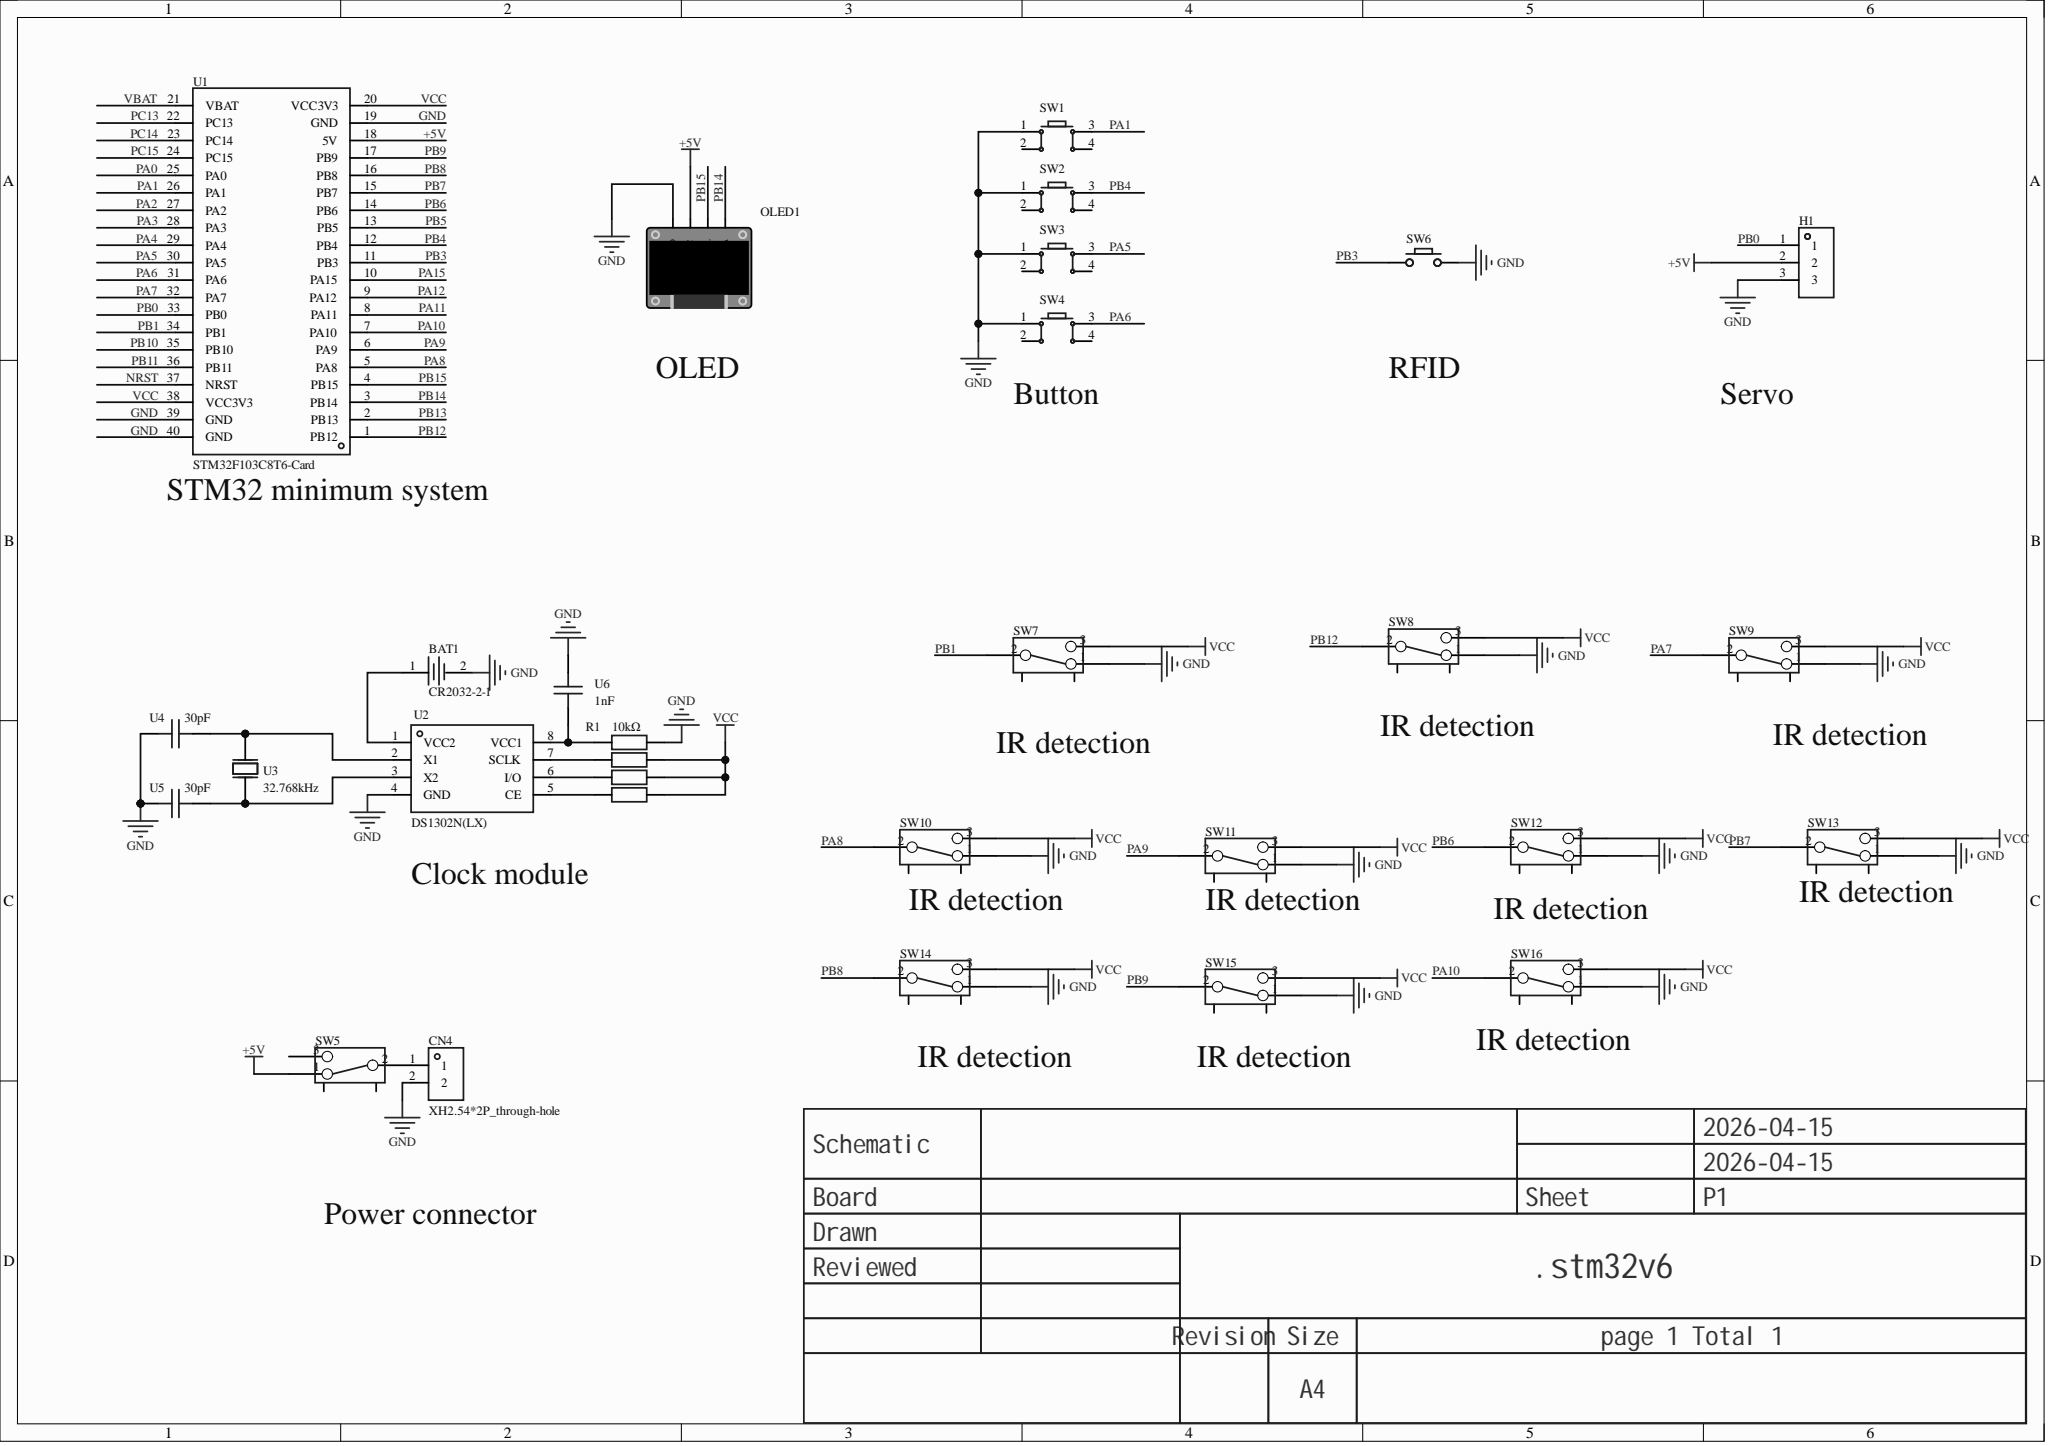Circuit board | Altium Designer | 30 parts | 29 nets
Bill of materials:
Comment,Description,Designator,Footprint,LibRef,Quantity
"CR2032-2-1","","BAT1","BAT-TH_CR2032-2-1","CR2032-2-1","1"
"XH2.54*2P_through-hole","","CN4","CONN-TH_2P-P2.50-XH2.54-2P","XH2.54*2P_直插","1"
"","","H1","HDR-TH_3P-P2.54-V-F","HDR-F_2.54_1x3P","1"
"","","OLED1","0.96OLED_4P","0.96OLED模块_4P","1"
"10kΩ","","R1, R2, R3, R4","Res_1/8W","Res_AXIAL-1/8W","4"
"","","SW1, SW2, SW3, SW4","SW-TH_4P-L6.0-W6.0-P4.50-LS6.5","Key_TH_6x6x6","4"
"","","SW5, SW7, SW8, SW9, SW10, SW11, SW12, SW13, SW14, SW15, SW16","拨动开关","拨动开关_正","11"
"","","SW6","Key_TH_3.5x6x4.3","Key_TH_3.5x6x4.3","1"
"STM32F103C8T6-Card","","U1","CONN-TH_L53.3-W22.9_STM32F103C8T6-CARD","STM32F103C8T6-Card","1"
"DS1302N(LX)","","U2","PDIP-8_L9.3-W6.4-P2.54-LS7.9-BL-1","DS1302N(LX)","1"
"32.768kHz","","U3","CRYSTAL-TH_BD2.1-P0.70-D0.3","C-002RX 32.768KHZ: PB FREE","1"
"30pF","","U4, U5","CAP-TH_L5.0-W2.5-P5.00-D1.0","100nF","2"
"1nF","","U6","CAP-TH_L5.0-W2.5-P5.00-D1.0","100nF","1"
Netlist (Protel format):
[
BAT1
BAT-TH_CR2032-2-1
CR2032-2-1



]
[
CN4
CONN-TH_2P-P2.50-XH2.54-2P
XH2.54*2P_through-hole



]
[
H1
HDR-TH_3P-P2.54-V-F




]
[
OLED1
0.96OLED_4P




]
[
R1
Res_1/8W
10kΩ



]
[
R2
Res_1/8W
10kΩ



]
[
R3
Res_1/8W
10kΩ



]
[
R4
Res_1/8W
10kΩ



]
[
SW1
SW-TH_4P-L6.0-W6.0-P4.50-LS6.5




]
[
SW2
SW-TH_4P-L6.0-W6.0-P4.50-LS6.5




]
[
SW3
SW-TH_4P-L6.0-W6.0-P4.50-LS6.5




]
[
SW4
SW-TH_4P-L6.0-W6.0-P4.50-LS6.5




]
[
SW5
拨动开关




]
[
SW6
Key_TH_3.5x6x4.3




]
[
SW7
拨动开关




]
[
SW8
拨动开关




]
[
SW9
拨动开关




]
[
SW10
拨动开关




]
[
SW11
拨动开关




]
[
SW12
拨动开关




]
[
SW13
拨动开关




]
[
SW14
拨动开关




]
[
SW15
拨动开关




]
[
SW16
拨动开关




]
[
U1
CONN-TH_L53.3-W22.9_STM32F103C8T6-CARD
STM32F103C8T6-Card



]
[
U2
PDIP-8_L9.3-W6.4-P2.54-LS7.9-BL-1
DS1302N(LX)



]
[
U3
CRYSTAL-TH_BD2.1-P0.70-D0.3
32.768kHz



]
[
U4
CAP-TH_L5.0-W2.5-P5.00-D1.0
30pF



]
[
U5
CAP-TH_L5.0-W2.5-P5.00-D1.0
30pF



]
[
U6
CAP-TH_L5.0-W2.5-P5.00-D1.0
1nF



]
(
VCC
R2-2
R3-2
R4-2
SW7-3
SW8-3
SW9-3
SW10-3
SW11-3
SW12-3
SW13-3
SW14-3
SW15-3
SW16-3
U1-20
U1-38
)
(
PB15
OLED1-3
U1-4
)
(
PB14
OLED1-4
U1-3
)
(
PB12
SW8-2
U1-1
)
(
PB9
SW15-2
U1-17
)
(
PB8
SW14-2
U1-16
)
(
PB7
SW13-2
U1-15
)
(
PB6
SW12-2
U1-14
)
(
PB4
SW2-3
U1-12
)
(
PB3
SW6-A
U1-11
)
(
PB1
SW7-2
U1-34
)
(
PB0
H1-1
U1-33
)
(
PA10
SW16-2
U1-7
)
(
PA9
SW11-2
U1-6
)
(
PA8
SW10-2
U1-5
)
(
PA7
SW9-2
U1-32
)
(
PA6
SW4-3
U1-31
)
(
PA5
SW3-3
U1-30
)
(
PA1
SW1-3
U1-26
)
(
NetU2_3
U2-3
U3-1
U5-1
)
(
NetU2_2
U2-2
U3-2
U4-1
)
(
NetR4_1
R4-1
U2-5
)
(
NetR3_1
R3-1
U2-6
)
(
NetR2_1
R2-1
U2-7
)
(
NetR1_1
R1-1
U2-8
U6-2
)
(
NetCN4_1
CN4-1
SW5-2
)
(
NetBAT1_1
BAT1-1
U2-1
)
(
GND
BAT1-2
CN4-2
H1-3
OLED1-1
R1-2
SW1-1
SW2-1
SW3-1
SW4-1
SW6-B
SW7-1
SW8-1
SW9-1
SW10-1
SW11-1
SW12-1
SW13-1
SW14-1
SW15-1
SW16-1
U1-19
U1-39
U1-40
U2-4
U4-2
U5-2
U6-1
)
(
+5V
H1-2
OLED1-2
SW5-1
U1-18
)